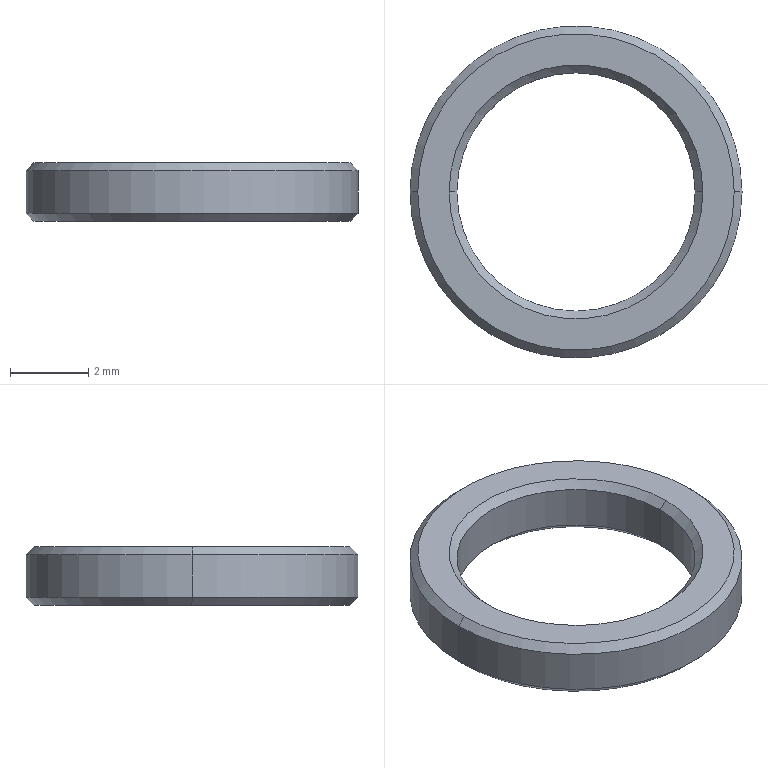Part | STEP file | 10000020559swp000-1 | 1 solid | 14 faces | box 8.5 x 8.5 x 1.5 mm | volume 39.446 mm3 | cone 8 | cylinder 4 | plane 2 | commonest cylinder face diameters 6.1 x2 8.5 x2
STEP:
#1=CARTESIAN_POINT('',(4.05,0.,1.5));
#2=VERTEX_POINT('',#1);
#3=CARTESIAN_POINT('',(-4.05,0.,1.5));
#4=VERTEX_POINT('',#3);
#5=CARTESIAN_POINT('',(0.,0.,1.5));
#6=DIRECTION('',(0.,0.,1.));
#7=DIRECTION('',(1.,0.,0.));
#8=AXIS2_PLACEMENT_3D('',#5,#6,#7);
#9=CIRCLE('',#8,4.05);
#10=EDGE_CURVE('',#2,#4,#9,.T.);
#11=ORIENTED_EDGE('',*,*,#10,.F.);
#12=CARTESIAN_POINT('',(4.25,0.,1.3));
#13=VERTEX_POINT('',#12);
#14=CARTESIAN_POINT('',(4.05,0.,1.5));
#15=DIRECTION('',(0.7071,0.,-0.7071));
#16=VECTOR('',#15,1000.);
#17=LINE('',#14,#16);
#18=EDGE_CURVE('',#2,#13,#17,.T.);
#19=ORIENTED_EDGE('',*,*,#18,.T.);
#20=CARTESIAN_POINT('',(-4.25,0.,1.3));
#21=VERTEX_POINT('',#20);
#22=CARTESIAN_POINT('',(0.,0.,1.3));
#23=DIRECTION('',(0.,0.,-1.));
#24=DIRECTION('',(1.,0.,0.));
#25=AXIS2_PLACEMENT_3D('',#22,#23,#24);
#26=CIRCLE('',#25,4.25);
#27=EDGE_CURVE('',#21,#13,#26,.T.);
#28=ORIENTED_EDGE('',*,*,#27,.F.);
#29=CARTESIAN_POINT('',(-4.05,0.,1.5));
#30=DIRECTION('',(-0.7071,0.,-0.7071));
#31=VECTOR('',#30,1000.);
#32=LINE('',#29,#31);
#33=EDGE_CURVE('',#4,#21,#32,.T.);
#34=ORIENTED_EDGE('',*,*,#33,.F.);
#35=EDGE_LOOP('',(#11,#19,#28,#34));
#36=FACE_OUTER_BOUND('',#35,.T.);
#37=CARTESIAN_POINT('',(0.,0.,1.5));
#38=DIRECTION('',(0.,0.,-1.));
#39=DIRECTION('',(-1.,0.,0.));
#40=AXIS2_PLACEMENT_3D('',#37,#38,#39);
#41=CONICAL_SURFACE('',#40,4.05,0.7854);
#42=ADVANCED_FACE('',(#36),#41,.T.);
#43=CARTESIAN_POINT('',(-4.05,0.,0.));
#44=VERTEX_POINT('',#43);
#45=CARTESIAN_POINT('',(4.05,0.,0.));
#46=VERTEX_POINT('',#45);
#47=CARTESIAN_POINT('',(0.,0.,0.));
#48=DIRECTION('',(0.,0.,-1.));
#49=DIRECTION('',(1.,0.,0.));
#50=AXIS2_PLACEMENT_3D('',#47,#48,#49);
#51=CIRCLE('',#50,4.05);
#52=EDGE_CURVE('',#44,#46,#51,.T.);
#53=ORIENTED_EDGE('',*,*,#52,.F.);
#54=CARTESIAN_POINT('',(-4.25,0.,0.2));
#55=VERTEX_POINT('',#54);
#56=CARTESIAN_POINT('',(-4.25,0.,0.2));
#57=DIRECTION('',(-0.7071,0.,0.7071));
#58=VECTOR('',#57,1000.);
#59=LINE('',#56,#58);
#60=EDGE_CURVE('',#44,#55,#59,.T.);
#61=ORIENTED_EDGE('',*,*,#60,.T.);
#62=CARTESIAN_POINT('',(4.25,0.,0.2));
#63=VERTEX_POINT('',#62);
#64=CARTESIAN_POINT('',(0.,0.,0.2));
#65=DIRECTION('',(0.,0.,1.));
#66=DIRECTION('',(1.,0.,0.));
#67=AXIS2_PLACEMENT_3D('',#64,#65,#66);
#68=CIRCLE('',#67,4.25);
#69=EDGE_CURVE('',#63,#55,#68,.T.);
#70=ORIENTED_EDGE('',*,*,#69,.F.);
#71=CARTESIAN_POINT('',(4.25,0.,0.2));
#72=DIRECTION('',(0.7071,0.,0.7071));
#73=VECTOR('',#72,1000.);
#74=LINE('',#71,#73);
#75=EDGE_CURVE('',#46,#63,#74,.T.);
#76=ORIENTED_EDGE('',*,*,#75,.F.);
#77=EDGE_LOOP('',(#53,#61,#70,#76));
#78=FACE_OUTER_BOUND('',#77,.T.);
#79=CARTESIAN_POINT('',(0.,0.,0.2));
#80=DIRECTION('',(0.,0.,1.));
#81=DIRECTION('',(1.,0.,0.));
#82=AXIS2_PLACEMENT_3D('',#79,#80,#81);
#83=CONICAL_SURFACE('',#82,4.25,0.7854);
#84=ADVANCED_FACE('',(#78),#83,.T.);
#85=CARTESIAN_POINT('',(-3.05,0.,1.3));
#86=VERTEX_POINT('',#85);
#87=CARTESIAN_POINT('',(3.05,0.,1.3));
#88=VERTEX_POINT('',#87);
#89=CARTESIAN_POINT('',(0.,0.,1.3));
#90=DIRECTION('',(0.,0.,1.));
#91=DIRECTION('',(1.,0.,0.));
#92=AXIS2_PLACEMENT_3D('',#89,#90,#91);
#93=CIRCLE('',#92,3.05);
#94=EDGE_CURVE('',#86,#88,#93,.T.);
#95=ORIENTED_EDGE('',*,*,#94,.F.);
#96=CARTESIAN_POINT('',(-3.25,0.,1.5));
#97=VERTEX_POINT('',#96);
#98=CARTESIAN_POINT('',(-3.05,0.,1.3));
#99=DIRECTION('',(-0.7071,0.,0.7071));
#100=VECTOR('',#99,1000.);
#101=LINE('',#98,#100);
#102=EDGE_CURVE('',#86,#97,#101,.T.);
#103=ORIENTED_EDGE('',*,*,#102,.T.);
#104=CARTESIAN_POINT('',(3.25,0.,1.5));
#105=VERTEX_POINT('',#104);
#106=CARTESIAN_POINT('',(0.,0.,1.5));
#107=DIRECTION('',(0.,0.,-1.));
#108=DIRECTION('',(1.,0.,0.));
#109=AXIS2_PLACEMENT_3D('',#106,#107,#108);
#110=CIRCLE('',#109,3.25);
#111=EDGE_CURVE('',#105,#97,#110,.T.);
#112=ORIENTED_EDGE('',*,*,#111,.F.);
#113=CARTESIAN_POINT('',(3.05,0.,1.3));
#114=DIRECTION('',(0.7071,0.,0.7071));
#115=VECTOR('',#114,1000.);
#116=LINE('',#113,#115);
#117=EDGE_CURVE('',#88,#105,#116,.T.);
#118=ORIENTED_EDGE('',*,*,#117,.F.);
#119=EDGE_LOOP('',(#95,#103,#112,#118));
#120=FACE_OUTER_BOUND('',#119,.T.);
#121=CARTESIAN_POINT('',(0.,0.,1.3));
#122=DIRECTION('',(0.,0.,1.));
#123=DIRECTION('',(1.,0.,0.));
#124=AXIS2_PLACEMENT_3D('',#121,#122,#123);
#125=CONICAL_SURFACE('',#124,3.05,0.7854);
#126=ADVANCED_FACE('',(#120),#125,.F.);
#127=CARTESIAN_POINT('',(3.05,0.,0.2));
#128=VERTEX_POINT('',#127);
#129=CARTESIAN_POINT('',(-3.05,0.,0.2));
#130=VERTEX_POINT('',#129);
#131=CARTESIAN_POINT('',(0.,0.,0.2));
#132=DIRECTION('',(0.,0.,-1.));
#133=DIRECTION('',(1.,0.,0.));
#134=AXIS2_PLACEMENT_3D('',#131,#132,#133);
#135=CIRCLE('',#134,3.05);
#136=EDGE_CURVE('',#128,#130,#135,.T.);
#137=ORIENTED_EDGE('',*,*,#136,.F.);
#138=CARTESIAN_POINT('',(3.25,0.,0.));
#139=VERTEX_POINT('',#138);
#140=CARTESIAN_POINT('',(3.25,0.,0.));
#141=DIRECTION('',(0.7071,0.,-0.7071));
#142=VECTOR('',#141,1000.);
#143=LINE('',#140,#142);
#144=EDGE_CURVE('',#128,#139,#143,.T.);
#145=ORIENTED_EDGE('',*,*,#144,.T.);
#146=CARTESIAN_POINT('',(-3.25,0.,0.));
#147=VERTEX_POINT('',#146);
#148=CARTESIAN_POINT('',(0.,0.,0.));
#149=DIRECTION('',(0.,0.,1.));
#150=DIRECTION('',(1.,0.,0.));
#151=AXIS2_PLACEMENT_3D('',#148,#149,#150);
#152=CIRCLE('',#151,3.25);
#153=EDGE_CURVE('',#147,#139,#152,.T.);
#154=ORIENTED_EDGE('',*,*,#153,.F.);
#155=CARTESIAN_POINT('',(-3.25,0.,0.));
#156=DIRECTION('',(-0.7071,0.,-0.7071));
#157=VECTOR('',#156,1000.);
#158=LINE('',#155,#157);
#159=EDGE_CURVE('',#130,#147,#158,.T.);
#160=ORIENTED_EDGE('',*,*,#159,.F.);
#161=EDGE_LOOP('',(#137,#145,#154,#160));
#162=FACE_OUTER_BOUND('',#161,.T.);
#163=CARTESIAN_POINT('',(0.,0.,0.));
#164=DIRECTION('',(0.,0.,-1.));
#165=DIRECTION('',(-1.,0.,0.));
#166=AXIS2_PLACEMENT_3D('',#163,#164,#165);
#167=CONICAL_SURFACE('',#166,3.25,0.7854);
#168=ADVANCED_FACE('',(#162),#167,.F.);
#169=ORIENTED_EDGE('',*,*,#94,.T.);
#170=CARTESIAN_POINT('',(3.05,0.,1.5));
#171=DIRECTION('',(0.,0.,-1.));
#172=VECTOR('',#171,1000.);
#173=LINE('',#170,#172);
#174=EDGE_CURVE('',#88,#128,#173,.T.);
#175=ORIENTED_EDGE('',*,*,#174,.T.);
#176=ORIENTED_EDGE('',*,*,#136,.T.);
#177=CARTESIAN_POINT('',(-3.05,0.,1.5));
#178=DIRECTION('',(0.,0.,-1.));
#179=VECTOR('',#178,1000.);
#180=LINE('',#177,#179);
#181=EDGE_CURVE('',#86,#130,#180,.T.);
#182=ORIENTED_EDGE('',*,*,#181,.F.);
#183=EDGE_LOOP('',(#169,#175,#176,#182));
#184=FACE_OUTER_BOUND('',#183,.T.);
#185=CARTESIAN_POINT('',(0.,0.,1.5));
#186=DIRECTION('',(0.,0.,-1.));
#187=DIRECTION('',(-1.,0.,0.));
#188=AXIS2_PLACEMENT_3D('',#185,#186,#187);
#189=CYLINDRICAL_SURFACE('',#188,3.05);
#190=ADVANCED_FACE('',(#184),#189,.F.);
#191=ORIENTED_EDGE('',*,*,#27,.T.);
#192=CARTESIAN_POINT('',(4.25,0.,1.5));
#193=DIRECTION('',(0.,0.,-1.));
#194=VECTOR('',#193,1000.);
#195=LINE('',#192,#194);
#196=EDGE_CURVE('',#13,#63,#195,.T.);
#197=ORIENTED_EDGE('',*,*,#196,.T.);
#198=ORIENTED_EDGE('',*,*,#69,.T.);
#199=CARTESIAN_POINT('',(-4.25,0.,1.5));
#200=DIRECTION('',(0.,0.,-1.));
#201=VECTOR('',#200,1000.);
#202=LINE('',#199,#201);
#203=EDGE_CURVE('',#21,#55,#202,.T.);
#204=ORIENTED_EDGE('',*,*,#203,.F.);
#205=EDGE_LOOP('',(#191,#197,#198,#204));
#206=FACE_OUTER_BOUND('',#205,.T.);
#207=CARTESIAN_POINT('',(0.,0.,1.5));
#208=DIRECTION('',(0.,0.,-1.));
#209=DIRECTION('',(-1.,0.,0.));
#210=AXIS2_PLACEMENT_3D('',#207,#208,#209);
#211=CYLINDRICAL_SURFACE('',#210,4.25);
#212=ADVANCED_FACE('',(#206),#211,.T.);
#213=ORIENTED_EDGE('',*,*,#111,.T.);
#214=CARTESIAN_POINT('',(0.,0.,1.5));
#215=DIRECTION('',(0.,0.,-1.));
#216=DIRECTION('',(1.,0.,0.));
#217=AXIS2_PLACEMENT_3D('',#214,#215,#216);
#218=CIRCLE('',#217,3.25);
#219=EDGE_CURVE('',#97,#105,#218,.T.);
#220=ORIENTED_EDGE('',*,*,#219,.T.);
#221=EDGE_LOOP('',(#213,#220));
#222=FACE_BOUND('',#221,.T.);
#223=CARTESIAN_POINT('',(0.,0.,1.5));
#224=DIRECTION('',(0.,0.,1.));
#225=DIRECTION('',(1.,0.,0.));
#226=AXIS2_PLACEMENT_3D('',#223,#224,#225);
#227=CIRCLE('',#226,4.05);
#228=EDGE_CURVE('',#4,#2,#227,.T.);
#229=ORIENTED_EDGE('',*,*,#228,.T.);
#230=ORIENTED_EDGE('',*,*,#10,.T.);
#231=EDGE_LOOP('',(#229,#230));
#232=FACE_OUTER_BOUND('',#231,.T.);
#233=CARTESIAN_POINT('',(0.,0.,1.5));
#234=DIRECTION('',(0.,0.,1.));
#235=DIRECTION('',(1.,0.,0.));
#236=AXIS2_PLACEMENT_3D('',#233,#234,#235);
#237=PLANE('',#236);
#238=ADVANCED_FACE('',(#222,#232),#237,.T.);
#239=ORIENTED_EDGE('',*,*,#153,.T.);
#240=CARTESIAN_POINT('',(0.,0.,0.));
#241=DIRECTION('',(0.,0.,1.));
#242=DIRECTION('',(1.,0.,0.));
#243=AXIS2_PLACEMENT_3D('',#240,#241,#242);
#244=CIRCLE('',#243,3.25);
#245=EDGE_CURVE('',#139,#147,#244,.T.);
#246=ORIENTED_EDGE('',*,*,#245,.T.);
#247=EDGE_LOOP('',(#239,#246));
#248=FACE_BOUND('',#247,.T.);
#249=CARTESIAN_POINT('',(0.,0.,0.));
#250=DIRECTION('',(0.,0.,-1.));
#251=DIRECTION('',(1.,0.,0.));
#252=AXIS2_PLACEMENT_3D('',#249,#250,#251);
#253=CIRCLE('',#252,4.05);
#254=EDGE_CURVE('',#46,#44,#253,.T.);
#255=ORIENTED_EDGE('',*,*,#254,.T.);
#256=ORIENTED_EDGE('',*,*,#52,.T.);
#257=EDGE_LOOP('',(#255,#256));
#258=FACE_OUTER_BOUND('',#257,.T.);
#259=CARTESIAN_POINT('',(0.,0.,0.));
#260=DIRECTION('',(0.,0.,1.));
#261=DIRECTION('',(1.,0.,0.));
#262=AXIS2_PLACEMENT_3D('',#259,#260,#261);
#263=PLANE('',#262);
#264=ADVANCED_FACE('',(#248,#258),#263,.F.);
#265=ORIENTED_EDGE('',*,*,#196,.F.);
#266=CARTESIAN_POINT('',(0.,0.,1.3));
#267=DIRECTION('',(0.,0.,-1.));
#268=DIRECTION('',(1.,0.,0.));
#269=AXIS2_PLACEMENT_3D('',#266,#267,#268);
#270=CIRCLE('',#269,4.25);
#271=EDGE_CURVE('',#13,#21,#270,.T.);
#272=ORIENTED_EDGE('',*,*,#271,.T.);
#273=ORIENTED_EDGE('',*,*,#203,.T.);
#274=CARTESIAN_POINT('',(0.,0.,0.2));
#275=DIRECTION('',(0.,0.,1.));
#276=DIRECTION('',(1.,0.,0.));
#277=AXIS2_PLACEMENT_3D('',#274,#275,#276);
#278=CIRCLE('',#277,4.25);
#279=EDGE_CURVE('',#55,#63,#278,.T.);
#280=ORIENTED_EDGE('',*,*,#279,.T.);
#281=EDGE_LOOP('',(#265,#272,#273,#280));
#282=FACE_OUTER_BOUND('',#281,.T.);
#283=CARTESIAN_POINT('',(0.,0.,1.5));
#284=DIRECTION('',(0.,0.,-1.));
#285=DIRECTION('',(-1.,0.,0.));
#286=AXIS2_PLACEMENT_3D('',#283,#284,#285);
#287=CYLINDRICAL_SURFACE('',#286,4.25);
#288=ADVANCED_FACE('',(#282),#287,.T.);
#289=ORIENTED_EDGE('',*,*,#174,.F.);
#290=CARTESIAN_POINT('',(0.,0.,1.3));
#291=DIRECTION('',(0.,0.,1.));
#292=DIRECTION('',(1.,0.,0.));
#293=AXIS2_PLACEMENT_3D('',#290,#291,#292);
#294=CIRCLE('',#293,3.05);
#295=EDGE_CURVE('',#88,#86,#294,.T.);
#296=ORIENTED_EDGE('',*,*,#295,.T.);
#297=ORIENTED_EDGE('',*,*,#181,.T.);
#298=CARTESIAN_POINT('',(0.,0.,0.2));
#299=DIRECTION('',(0.,0.,-1.));
#300=DIRECTION('',(1.,0.,0.));
#301=AXIS2_PLACEMENT_3D('',#298,#299,#300);
#302=CIRCLE('',#301,3.05);
#303=EDGE_CURVE('',#130,#128,#302,.T.);
#304=ORIENTED_EDGE('',*,*,#303,.T.);
#305=EDGE_LOOP('',(#289,#296,#297,#304));
#306=FACE_OUTER_BOUND('',#305,.T.);
#307=CARTESIAN_POINT('',(0.,0.,1.5));
#308=DIRECTION('',(0.,0.,-1.));
#309=DIRECTION('',(-1.,0.,0.));
#310=AXIS2_PLACEMENT_3D('',#307,#308,#309);
#311=CYLINDRICAL_SURFACE('',#310,3.05);
#312=ADVANCED_FACE('',(#306),#311,.F.);
#313=ORIENTED_EDGE('',*,*,#144,.F.);
#314=ORIENTED_EDGE('',*,*,#303,.F.);
#315=ORIENTED_EDGE('',*,*,#159,.T.);
#316=ORIENTED_EDGE('',*,*,#245,.F.);
#317=EDGE_LOOP('',(#313,#314,#315,#316));
#318=FACE_OUTER_BOUND('',#317,.T.);
#319=CARTESIAN_POINT('',(0.,0.,0.));
#320=DIRECTION('',(0.,0.,-1.));
#321=DIRECTION('',(-1.,0.,0.));
#322=AXIS2_PLACEMENT_3D('',#319,#320,#321);
#323=CONICAL_SURFACE('',#322,3.25,0.7854);
#324=ADVANCED_FACE('',(#318),#323,.F.);
#325=ORIENTED_EDGE('',*,*,#102,.F.);
#326=ORIENTED_EDGE('',*,*,#295,.F.);
#327=ORIENTED_EDGE('',*,*,#117,.T.);
#328=ORIENTED_EDGE('',*,*,#219,.F.);
#329=EDGE_LOOP('',(#325,#326,#327,#328));
#330=FACE_OUTER_BOUND('',#329,.T.);
#331=CARTESIAN_POINT('',(0.,0.,1.3));
#332=DIRECTION('',(0.,0.,1.));
#333=DIRECTION('',(1.,0.,0.));
#334=AXIS2_PLACEMENT_3D('',#331,#332,#333);
#335=CONICAL_SURFACE('',#334,3.05,0.7854);
#336=ADVANCED_FACE('',(#330),#335,.F.);
#337=ORIENTED_EDGE('',*,*,#60,.F.);
#338=ORIENTED_EDGE('',*,*,#254,.F.);
#339=ORIENTED_EDGE('',*,*,#75,.T.);
#340=ORIENTED_EDGE('',*,*,#279,.F.);
#341=EDGE_LOOP('',(#337,#338,#339,#340));
#342=FACE_OUTER_BOUND('',#341,.T.);
#343=CARTESIAN_POINT('',(0.,0.,0.2));
#344=DIRECTION('',(0.,0.,1.));
#345=DIRECTION('',(1.,0.,0.));
#346=AXIS2_PLACEMENT_3D('',#343,#344,#345);
#347=CONICAL_SURFACE('',#346,4.25,0.7854);
#348=ADVANCED_FACE('',(#342),#347,.T.);
#349=ORIENTED_EDGE('',*,*,#18,.F.);
#350=ORIENTED_EDGE('',*,*,#228,.F.);
#351=ORIENTED_EDGE('',*,*,#33,.T.);
#352=ORIENTED_EDGE('',*,*,#271,.F.);
#353=EDGE_LOOP('',(#349,#350,#351,#352));
#354=FACE_OUTER_BOUND('',#353,.T.);
#355=CARTESIAN_POINT('',(0.,0.,1.5));
#356=DIRECTION('',(0.,0.,-1.));
#357=DIRECTION('',(-1.,0.,0.));
#358=AXIS2_PLACEMENT_3D('',#355,#356,#357);
#359=CONICAL_SURFACE('',#358,4.05,0.7854);
#360=ADVANCED_FACE('',(#354),#359,.T.);
#361=CLOSED_SHELL('',(#42,#84,#126,#168,#190,#212,#238,#264,#288,#312,#324,#336,#348,#360));
#362=MANIFOLD_SOLID_BREP('',#361);
#363=CARTESIAN_POINT('',(0.,0.,0.));
#364=DIRECTION('',(0.,0.,1.));
#365=DIRECTION('',(1.,0.,0.));
#366=AXIS2_PLACEMENT_3D('',#363,#364,#365);
#367=(LENGTH_UNIT()NAMED_UNIT(*)SI_UNIT(.MILLI.,.METRE.));
#368=UNCERTAINTY_MEASURE_WITH_UNIT(LENGTH_MEASURE(0.00001),#367,'','');
#369=(NAMED_UNIT(*)PLANE_ANGLE_UNIT()SI_UNIT($,.RADIAN.));
#370=(NAMED_UNIT(*)SI_UNIT($,.STERADIAN.)SOLID_ANGLE_UNIT());
#371=(GEOMETRIC_REPRESENTATION_CONTEXT(3)GLOBAL_UNCERTAINTY_ASSIGNED_CONTEXT((#368))GLOBAL_UNIT_ASSIGNED_CONTEXT((#367,#369,#370))REPRESENTATION_CONTEXT('',''));
#372=ADVANCED_BREP_SHAPE_REPRESENTATION('',(#362,#366),#371);